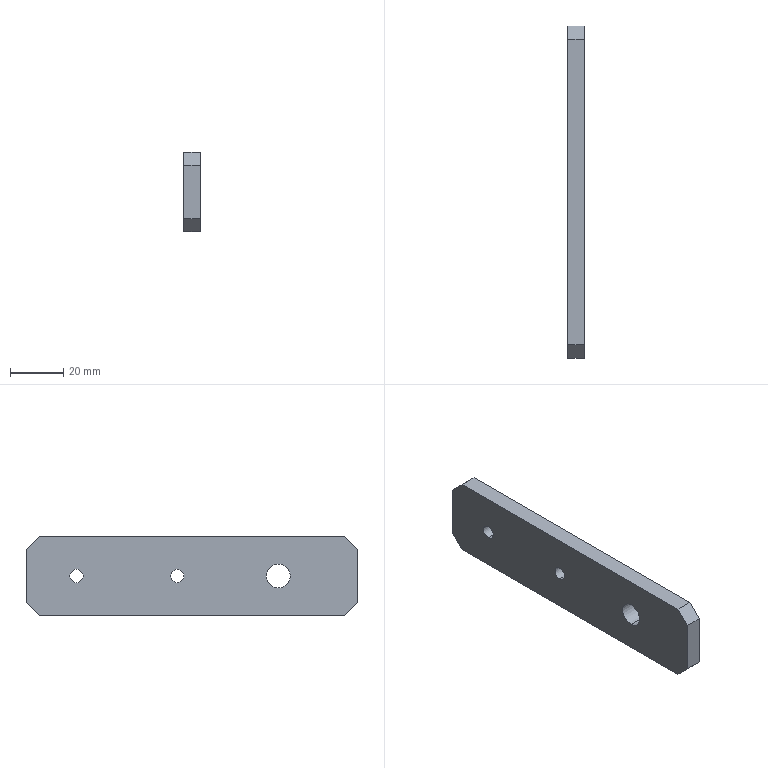Part | STEP file | PLACA SOPORTE GUIA | 1 solid | 16 faces | box 6.35 x 125 x 30 mm | volume 22842 mm3 | plane 10 | cylinder 6 | commonest cylinder face diameters 5 x4 9 x2
STEP:
#1=CARTESIAN_POINT('',(6.35,43.5,-2.5));
#2=VERTEX_POINT('',#1);
#3=CARTESIAN_POINT('',(6.35,43.5,2.5));
#4=VERTEX_POINT('',#3);
#5=CARTESIAN_POINT('',(6.35,43.5,0.));
#6=DIRECTION('',(-1.,0.,0.));
#7=DIRECTION('',(0.,0.,1.));
#8=AXIS2_PLACEMENT_3D('',#5,#6,#7);
#9=CIRCLE('',#8,2.5);
#10=EDGE_CURVE('',#2,#4,#9,.T.);
#11=ORIENTED_EDGE('',*,*,#10,.F.);
#12=CARTESIAN_POINT('',(0.,43.5,-2.5));
#13=VERTEX_POINT('',#12);
#14=CARTESIAN_POINT('',(0.,43.5,-2.5));
#15=DIRECTION('',(-1.,0.,0.));
#16=VECTOR('',#15,1000.);
#17=LINE('',#14,#16);
#18=EDGE_CURVE('',#2,#13,#17,.T.);
#19=ORIENTED_EDGE('',*,*,#18,.T.);
#20=CARTESIAN_POINT('',(0.,43.5,2.5));
#21=VERTEX_POINT('',#20);
#22=CARTESIAN_POINT('',(0.,43.5,0.));
#23=DIRECTION('',(-1.,0.,0.));
#24=DIRECTION('',(0.,0.,1.));
#25=AXIS2_PLACEMENT_3D('',#22,#23,#24);
#26=CIRCLE('',#25,2.5);
#27=EDGE_CURVE('',#13,#21,#26,.T.);
#28=ORIENTED_EDGE('',*,*,#27,.T.);
#29=CARTESIAN_POINT('',(0.,43.5,2.5));
#30=DIRECTION('',(-1.,0.,0.));
#31=VECTOR('',#30,1000.);
#32=LINE('',#29,#31);
#33=EDGE_CURVE('',#4,#21,#32,.T.);
#34=ORIENTED_EDGE('',*,*,#33,.F.);
#35=EDGE_LOOP('',(#11,#19,#28,#34));
#36=FACE_OUTER_BOUND('',#35,.T.);
#37=CARTESIAN_POINT('',(0.,43.5,0.));
#38=DIRECTION('',(-1.,0.,0.));
#39=DIRECTION('',(0.,0.,1.));
#40=AXIS2_PLACEMENT_3D('',#37,#38,#39);
#41=CYLINDRICAL_SURFACE('',#40,2.5);
#42=ADVANCED_FACE('',(#36),#41,.F.);
#43=CARTESIAN_POINT('',(6.35,5.5,-2.5));
#44=VERTEX_POINT('',#43);
#45=CARTESIAN_POINT('',(6.35,5.5,2.5));
#46=VERTEX_POINT('',#45);
#47=CARTESIAN_POINT('',(6.35,5.5,0.));
#48=DIRECTION('',(-1.,0.,0.));
#49=DIRECTION('',(0.,0.,1.));
#50=AXIS2_PLACEMENT_3D('',#47,#48,#49);
#51=CIRCLE('',#50,2.5);
#52=EDGE_CURVE('',#44,#46,#51,.T.);
#53=ORIENTED_EDGE('',*,*,#52,.F.);
#54=CARTESIAN_POINT('',(0.,5.5,-2.5));
#55=VERTEX_POINT('',#54);
#56=CARTESIAN_POINT('',(0.,5.5,-2.5));
#57=DIRECTION('',(-1.,0.,0.));
#58=VECTOR('',#57,1000.);
#59=LINE('',#56,#58);
#60=EDGE_CURVE('',#44,#55,#59,.T.);
#61=ORIENTED_EDGE('',*,*,#60,.T.);
#62=CARTESIAN_POINT('',(0.,5.5,2.5));
#63=VERTEX_POINT('',#62);
#64=CARTESIAN_POINT('',(0.,5.5,0.));
#65=DIRECTION('',(-1.,0.,0.));
#66=DIRECTION('',(0.,0.,1.));
#67=AXIS2_PLACEMENT_3D('',#64,#65,#66);
#68=CIRCLE('',#67,2.5);
#69=EDGE_CURVE('',#55,#63,#68,.T.);
#70=ORIENTED_EDGE('',*,*,#69,.T.);
#71=CARTESIAN_POINT('',(0.,5.5,2.5));
#72=DIRECTION('',(-1.,0.,0.));
#73=VECTOR('',#72,1000.);
#74=LINE('',#71,#73);
#75=EDGE_CURVE('',#46,#63,#74,.T.);
#76=ORIENTED_EDGE('',*,*,#75,.F.);
#77=EDGE_LOOP('',(#53,#61,#70,#76));
#78=FACE_OUTER_BOUND('',#77,.T.);
#79=CARTESIAN_POINT('',(0.,5.5,0.));
#80=DIRECTION('',(-1.,0.,0.));
#81=DIRECTION('',(0.,0.,1.));
#82=AXIS2_PLACEMENT_3D('',#79,#80,#81);
#83=CYLINDRICAL_SURFACE('',#82,2.5);
#84=ADVANCED_FACE('',(#78),#83,.F.);
#85=CARTESIAN_POINT('',(6.35,-32.5,-4.5));
#86=VERTEX_POINT('',#85);
#87=CARTESIAN_POINT('',(6.35,-32.5,4.5));
#88=VERTEX_POINT('',#87);
#89=CARTESIAN_POINT('',(6.35,-32.5,0.));
#90=DIRECTION('',(-1.,0.,0.));
#91=DIRECTION('',(0.,0.,1.));
#92=AXIS2_PLACEMENT_3D('',#89,#90,#91);
#93=CIRCLE('',#92,4.5);
#94=EDGE_CURVE('',#86,#88,#93,.T.);
#95=ORIENTED_EDGE('',*,*,#94,.F.);
#96=CARTESIAN_POINT('',(0.,-32.5,-4.5));
#97=VERTEX_POINT('',#96);
#98=CARTESIAN_POINT('',(0.,-32.5,-4.5));
#99=DIRECTION('',(-1.,0.,0.));
#100=VECTOR('',#99,1000.);
#101=LINE('',#98,#100);
#102=EDGE_CURVE('',#86,#97,#101,.T.);
#103=ORIENTED_EDGE('',*,*,#102,.T.);
#104=CARTESIAN_POINT('',(0.,-32.5,4.5));
#105=VERTEX_POINT('',#104);
#106=CARTESIAN_POINT('',(0.,-32.5,0.));
#107=DIRECTION('',(-1.,0.,0.));
#108=DIRECTION('',(0.,0.,1.));
#109=AXIS2_PLACEMENT_3D('',#106,#107,#108);
#110=CIRCLE('',#109,4.5);
#111=EDGE_CURVE('',#97,#105,#110,.T.);
#112=ORIENTED_EDGE('',*,*,#111,.T.);
#113=CARTESIAN_POINT('',(0.,-32.5,4.5));
#114=DIRECTION('',(-1.,0.,0.));
#115=VECTOR('',#114,1000.);
#116=LINE('',#113,#115);
#117=EDGE_CURVE('',#88,#105,#116,.T.);
#118=ORIENTED_EDGE('',*,*,#117,.F.);
#119=EDGE_LOOP('',(#95,#103,#112,#118));
#120=FACE_OUTER_BOUND('',#119,.T.);
#121=CARTESIAN_POINT('',(0.,-32.5,0.));
#122=DIRECTION('',(-1.,0.,0.));
#123=DIRECTION('',(0.,0.,1.));
#124=AXIS2_PLACEMENT_3D('',#121,#122,#123);
#125=CYLINDRICAL_SURFACE('',#124,4.5);
#126=ADVANCED_FACE('',(#120),#125,.F.);
#127=CARTESIAN_POINT('',(6.35,-57.5,-15.));
#128=VERTEX_POINT('',#127);
#129=CARTESIAN_POINT('',(6.35,57.5,-15.));
#130=VERTEX_POINT('',#129);
#131=CARTESIAN_POINT('',(6.35,62.5,-15.));
#132=DIRECTION('',(0.,1.,0.));
#133=VECTOR('',#132,1000.);
#134=LINE('',#131,#133);
#135=EDGE_CURVE('',#128,#130,#134,.T.);
#136=ORIENTED_EDGE('',*,*,#135,.F.);
#137=CARTESIAN_POINT('',(0.,-57.5,-15.));
#138=VERTEX_POINT('',#137);
#139=CARTESIAN_POINT('',(6.35,-57.5,-15.));
#140=DIRECTION('',(-1.,0.,0.));
#141=VECTOR('',#140,1000.);
#142=LINE('',#139,#141);
#143=EDGE_CURVE('',#128,#138,#142,.T.);
#144=ORIENTED_EDGE('',*,*,#143,.T.);
#145=CARTESIAN_POINT('',(0.,57.5,-15.));
#146=VERTEX_POINT('',#145);
#147=CARTESIAN_POINT('',(0.,62.5,-15.));
#148=DIRECTION('',(0.,1.,0.));
#149=VECTOR('',#148,1000.);
#150=LINE('',#147,#149);
#151=EDGE_CURVE('',#138,#146,#150,.T.);
#152=ORIENTED_EDGE('',*,*,#151,.T.);
#153=CARTESIAN_POINT('',(6.35,57.5,-15.));
#154=DIRECTION('',(1.,0.,0.));
#155=VECTOR('',#154,1000.);
#156=LINE('',#153,#155);
#157=EDGE_CURVE('',#146,#130,#156,.T.);
#158=ORIENTED_EDGE('',*,*,#157,.T.);
#159=EDGE_LOOP('',(#136,#144,#152,#158));
#160=FACE_OUTER_BOUND('',#159,.T.);
#161=CARTESIAN_POINT('',(6.35,62.5,-15.));
#162=DIRECTION('',(0.,0.,1.));
#163=DIRECTION('',(0.,-1.,0.));
#164=AXIS2_PLACEMENT_3D('',#161,#162,#163);
#165=PLANE('',#164);
#166=ADVANCED_FACE('',(#160),#165,.F.);
#167=CARTESIAN_POINT('',(6.35,62.5,-10.));
#168=VERTEX_POINT('',#167);
#169=CARTESIAN_POINT('',(6.35,62.5,10.));
#170=VERTEX_POINT('',#169);
#171=CARTESIAN_POINT('',(6.35,62.5,15.));
#172=DIRECTION('',(0.,0.,1.));
#173=VECTOR('',#172,1000.);
#174=LINE('',#171,#173);
#175=EDGE_CURVE('',#168,#170,#174,.T.);
#176=ORIENTED_EDGE('',*,*,#175,.F.);
#177=CARTESIAN_POINT('',(0.,62.5,-10.));
#178=VERTEX_POINT('',#177);
#179=CARTESIAN_POINT('',(6.35,62.5,-10.));
#180=DIRECTION('',(-1.,0.,0.));
#181=VECTOR('',#180,1000.);
#182=LINE('',#179,#181);
#183=EDGE_CURVE('',#168,#178,#182,.T.);
#184=ORIENTED_EDGE('',*,*,#183,.T.);
#185=CARTESIAN_POINT('',(0.,62.5,10.));
#186=VERTEX_POINT('',#185);
#187=CARTESIAN_POINT('',(0.,62.5,15.));
#188=DIRECTION('',(0.,0.,1.));
#189=VECTOR('',#188,1000.);
#190=LINE('',#187,#189);
#191=EDGE_CURVE('',#178,#186,#190,.T.);
#192=ORIENTED_EDGE('',*,*,#191,.T.);
#193=CARTESIAN_POINT('',(6.35,62.5,10.));
#194=DIRECTION('',(1.,0.,0.));
#195=VECTOR('',#194,1000.);
#196=LINE('',#193,#195);
#197=EDGE_CURVE('',#186,#170,#196,.T.);
#198=ORIENTED_EDGE('',*,*,#197,.T.);
#199=EDGE_LOOP('',(#176,#184,#192,#198));
#200=FACE_OUTER_BOUND('',#199,.T.);
#201=CARTESIAN_POINT('',(6.35,62.5,15.));
#202=DIRECTION('',(0.,-1.,0.));
#203=DIRECTION('',(0.,0.,-1.));
#204=AXIS2_PLACEMENT_3D('',#201,#202,#203);
#205=PLANE('',#204);
#206=ADVANCED_FACE('',(#200),#205,.F.);
#207=CARTESIAN_POINT('',(0.,57.5,15.));
#208=VERTEX_POINT('',#207);
#209=CARTESIAN_POINT('',(0.,-57.5,15.));
#210=VERTEX_POINT('',#209);
#211=CARTESIAN_POINT('',(0.,62.5,15.));
#212=DIRECTION('',(0.,-1.,0.));
#213=VECTOR('',#212,1000.);
#214=LINE('',#211,#213);
#215=EDGE_CURVE('',#208,#210,#214,.T.);
#216=ORIENTED_EDGE('',*,*,#215,.T.);
#217=CARTESIAN_POINT('',(6.35,-57.5,15.));
#218=VERTEX_POINT('',#217);
#219=CARTESIAN_POINT('',(6.35,-57.5,15.));
#220=DIRECTION('',(1.,0.,0.));
#221=VECTOR('',#220,1000.);
#222=LINE('',#219,#221);
#223=EDGE_CURVE('',#210,#218,#222,.T.);
#224=ORIENTED_EDGE('',*,*,#223,.T.);
#225=CARTESIAN_POINT('',(6.35,57.5,15.));
#226=VERTEX_POINT('',#225);
#227=CARTESIAN_POINT('',(6.35,62.5,15.));
#228=DIRECTION('',(0.,-1.,0.));
#229=VECTOR('',#228,1000.);
#230=LINE('',#227,#229);
#231=EDGE_CURVE('',#226,#218,#230,.T.);
#232=ORIENTED_EDGE('',*,*,#231,.F.);
#233=CARTESIAN_POINT('',(6.35,57.5,15.));
#234=DIRECTION('',(-1.,0.,0.));
#235=VECTOR('',#234,1000.);
#236=LINE('',#233,#235);
#237=EDGE_CURVE('',#226,#208,#236,.T.);
#238=ORIENTED_EDGE('',*,*,#237,.T.);
#239=EDGE_LOOP('',(#216,#224,#232,#238));
#240=FACE_OUTER_BOUND('',#239,.T.);
#241=CARTESIAN_POINT('',(6.35,62.5,15.));
#242=DIRECTION('',(0.,0.,-1.));
#243=DIRECTION('',(0.,1.,0.));
#244=AXIS2_PLACEMENT_3D('',#241,#242,#243);
#245=PLANE('',#244);
#246=ADVANCED_FACE('',(#240),#245,.F.);
#247=CARTESIAN_POINT('',(0.,-62.5,10.));
#248=VERTEX_POINT('',#247);
#249=CARTESIAN_POINT('',(0.,-62.5,-10.));
#250=VERTEX_POINT('',#249);
#251=CARTESIAN_POINT('',(0.,-62.5,15.));
#252=DIRECTION('',(0.,0.,-1.));
#253=VECTOR('',#252,1000.);
#254=LINE('',#251,#253);
#255=EDGE_CURVE('',#248,#250,#254,.T.);
#256=ORIENTED_EDGE('',*,*,#255,.T.);
#257=CARTESIAN_POINT('',(6.35,-62.5,-10.));
#258=VERTEX_POINT('',#257);
#259=CARTESIAN_POINT('',(6.35,-62.5,-10.));
#260=DIRECTION('',(1.,0.,0.));
#261=VECTOR('',#260,1000.);
#262=LINE('',#259,#261);
#263=EDGE_CURVE('',#250,#258,#262,.T.);
#264=ORIENTED_EDGE('',*,*,#263,.T.);
#265=CARTESIAN_POINT('',(6.35,-62.5,10.));
#266=VERTEX_POINT('',#265);
#267=CARTESIAN_POINT('',(6.35,-62.5,15.));
#268=DIRECTION('',(0.,0.,-1.));
#269=VECTOR('',#268,1000.);
#270=LINE('',#267,#269);
#271=EDGE_CURVE('',#266,#258,#270,.T.);
#272=ORIENTED_EDGE('',*,*,#271,.F.);
#273=CARTESIAN_POINT('',(6.35,-62.5,10.));
#274=DIRECTION('',(-1.,0.,0.));
#275=VECTOR('',#274,1000.);
#276=LINE('',#273,#275);
#277=EDGE_CURVE('',#266,#248,#276,.T.);
#278=ORIENTED_EDGE('',*,*,#277,.T.);
#279=EDGE_LOOP('',(#256,#264,#272,#278));
#280=FACE_OUTER_BOUND('',#279,.T.);
#281=CARTESIAN_POINT('',(6.35,-62.5,15.));
#282=DIRECTION('',(0.,1.,0.));
#283=DIRECTION('',(0.,0.,1.));
#284=AXIS2_PLACEMENT_3D('',#281,#282,#283);
#285=PLANE('',#284);
#286=ADVANCED_FACE('',(#280),#285,.F.);
#287=CARTESIAN_POINT('',(6.35,43.5,0.));
#288=DIRECTION('',(-1.,0.,0.));
#289=DIRECTION('',(0.,0.,1.));
#290=AXIS2_PLACEMENT_3D('',#287,#288,#289);
#291=CIRCLE('',#290,2.5);
#292=EDGE_CURVE('',#4,#2,#291,.T.);
#293=ORIENTED_EDGE('',*,*,#292,.T.);
#294=ORIENTED_EDGE('',*,*,#10,.T.);
#295=EDGE_LOOP('',(#293,#294));
#296=FACE_BOUND('',#295,.T.);
#297=CARTESIAN_POINT('',(6.35,5.5,0.));
#298=DIRECTION('',(-1.,0.,0.));
#299=DIRECTION('',(0.,0.,1.));
#300=AXIS2_PLACEMENT_3D('',#297,#298,#299);
#301=CIRCLE('',#300,2.5);
#302=EDGE_CURVE('',#46,#44,#301,.T.);
#303=ORIENTED_EDGE('',*,*,#302,.T.);
#304=ORIENTED_EDGE('',*,*,#52,.T.);
#305=EDGE_LOOP('',(#303,#304));
#306=FACE_BOUND('',#305,.T.);
#307=CARTESIAN_POINT('',(6.35,-32.5,0.));
#308=DIRECTION('',(-1.,0.,0.));
#309=DIRECTION('',(0.,0.,1.));
#310=AXIS2_PLACEMENT_3D('',#307,#308,#309);
#311=CIRCLE('',#310,4.5);
#312=EDGE_CURVE('',#88,#86,#311,.T.);
#313=ORIENTED_EDGE('',*,*,#312,.T.);
#314=ORIENTED_EDGE('',*,*,#94,.T.);
#315=EDGE_LOOP('',(#313,#314));
#316=FACE_BOUND('',#315,.T.);
#317=ORIENTED_EDGE('',*,*,#271,.T.);
#318=CARTESIAN_POINT('',(6.35,-36.25,-36.25));
#319=DIRECTION('',(0.,0.7071,-0.7071));
#320=VECTOR('',#319,1000.);
#321=LINE('',#318,#320);
#322=EDGE_CURVE('',#258,#128,#321,.T.);
#323=ORIENTED_EDGE('',*,*,#322,.T.);
#324=ORIENTED_EDGE('',*,*,#135,.T.);
#325=CARTESIAN_POINT('',(6.35,36.25,-36.25));
#326=DIRECTION('',(0.,0.7071,0.7071));
#327=VECTOR('',#326,1000.);
#328=LINE('',#325,#327);
#329=EDGE_CURVE('',#130,#168,#328,.T.);
#330=ORIENTED_EDGE('',*,*,#329,.T.);
#331=ORIENTED_EDGE('',*,*,#175,.T.);
#332=CARTESIAN_POINT('',(6.35,36.25,36.25));
#333=DIRECTION('',(0.,-0.7071,0.7071));
#334=VECTOR('',#333,1000.);
#335=LINE('',#332,#334);
#336=EDGE_CURVE('',#170,#226,#335,.T.);
#337=ORIENTED_EDGE('',*,*,#336,.T.);
#338=ORIENTED_EDGE('',*,*,#231,.T.);
#339=CARTESIAN_POINT('',(6.35,-36.25,36.25));
#340=DIRECTION('',(0.,-0.7071,-0.7071));
#341=VECTOR('',#340,1000.);
#342=LINE('',#339,#341);
#343=EDGE_CURVE('',#218,#266,#342,.T.);
#344=ORIENTED_EDGE('',*,*,#343,.T.);
#345=EDGE_LOOP('',(#317,#323,#324,#330,#331,#337,#338,#344));
#346=FACE_OUTER_BOUND('',#345,.T.);
#347=CARTESIAN_POINT('',(6.35,0.,0.));
#348=DIRECTION('',(1.,0.,0.));
#349=DIRECTION('',(0.,0.,-1.));
#350=AXIS2_PLACEMENT_3D('',#347,#348,#349);
#351=PLANE('',#350);
#352=ADVANCED_FACE('',(#296,#306,#316,#346),#351,.T.);
#353=CARTESIAN_POINT('',(0.,43.5,0.));
#354=DIRECTION('',(-1.,0.,0.));
#355=DIRECTION('',(0.,0.,1.));
#356=AXIS2_PLACEMENT_3D('',#353,#354,#355);
#357=CIRCLE('',#356,2.5);
#358=EDGE_CURVE('',#21,#13,#357,.T.);
#359=ORIENTED_EDGE('',*,*,#358,.F.);
#360=ORIENTED_EDGE('',*,*,#27,.F.);
#361=EDGE_LOOP('',(#359,#360));
#362=FACE_BOUND('',#361,.T.);
#363=CARTESIAN_POINT('',(0.,5.5,0.));
#364=DIRECTION('',(-1.,0.,0.));
#365=DIRECTION('',(0.,0.,1.));
#366=AXIS2_PLACEMENT_3D('',#363,#364,#365);
#367=CIRCLE('',#366,2.5);
#368=EDGE_CURVE('',#63,#55,#367,.T.);
#369=ORIENTED_EDGE('',*,*,#368,.F.);
#370=ORIENTED_EDGE('',*,*,#69,.F.);
#371=EDGE_LOOP('',(#369,#370));
#372=FACE_BOUND('',#371,.T.);
#373=CARTESIAN_POINT('',(0.,-32.5,0.));
#374=DIRECTION('',(-1.,0.,0.));
#375=DIRECTION('',(0.,0.,1.));
#376=AXIS2_PLACEMENT_3D('',#373,#374,#375);
#377=CIRCLE('',#376,4.5);
#378=EDGE_CURVE('',#105,#97,#377,.T.);
#379=ORIENTED_EDGE('',*,*,#378,.F.);
#380=ORIENTED_EDGE('',*,*,#111,.F.);
#381=EDGE_LOOP('',(#379,#380));
#382=FACE_BOUND('',#381,.T.);
#383=ORIENTED_EDGE('',*,*,#151,.F.);
#384=CARTESIAN_POINT('',(0.,-57.5,-15.));
#385=DIRECTION('',(0.,-0.7071,0.7071));
#386=VECTOR('',#385,1000.);
#387=LINE('',#384,#386);
#388=EDGE_CURVE('',#138,#250,#387,.T.);
#389=ORIENTED_EDGE('',*,*,#388,.T.);
#390=ORIENTED_EDGE('',*,*,#255,.F.);
#391=CARTESIAN_POINT('',(0.,-62.5,10.));
#392=DIRECTION('',(0.,0.7071,0.7071));
#393=VECTOR('',#392,1000.);
#394=LINE('',#391,#393);
#395=EDGE_CURVE('',#248,#210,#394,.T.);
#396=ORIENTED_EDGE('',*,*,#395,.T.);
#397=ORIENTED_EDGE('',*,*,#215,.F.);
#398=CARTESIAN_POINT('',(0.,57.5,15.));
#399=DIRECTION('',(0.,0.7071,-0.7071));
#400=VECTOR('',#399,1000.);
#401=LINE('',#398,#400);
#402=EDGE_CURVE('',#208,#186,#401,.T.);
#403=ORIENTED_EDGE('',*,*,#402,.T.);
#404=ORIENTED_EDGE('',*,*,#191,.F.);
#405=CARTESIAN_POINT('',(0.,62.5,-10.));
#406=DIRECTION('',(0.,-0.7071,-0.7071));
#407=VECTOR('',#406,1000.);
#408=LINE('',#405,#407);
#409=EDGE_CURVE('',#178,#146,#408,.T.);
#410=ORIENTED_EDGE('',*,*,#409,.T.);
#411=EDGE_LOOP('',(#383,#389,#390,#396,#397,#403,#404,#410));
#412=FACE_OUTER_BOUND('',#411,.T.);
#413=CARTESIAN_POINT('',(0.,0.,0.));
#414=DIRECTION('',(1.,0.,0.));
#415=DIRECTION('',(0.,0.,-1.));
#416=AXIS2_PLACEMENT_3D('',#413,#414,#415);
#417=PLANE('',#416);
#418=ADVANCED_FACE('',(#362,#372,#382,#412),#417,.F.);
#419=ORIENTED_EDGE('',*,*,#322,.F.);
#420=ORIENTED_EDGE('',*,*,#263,.F.);
#421=ORIENTED_EDGE('',*,*,#388,.F.);
#422=ORIENTED_EDGE('',*,*,#143,.F.);
#423=EDGE_LOOP('',(#419,#420,#421,#422));
#424=FACE_OUTER_BOUND('',#423,.T.);
#425=CARTESIAN_POINT('',(6.35,-57.5,-15.));
#426=DIRECTION('',(0.,0.7071,0.7071));
#427=DIRECTION('',(-1.,0.,0.));
#428=AXIS2_PLACEMENT_3D('',#425,#426,#427);
#429=PLANE('',#428);
#430=ADVANCED_FACE('',(#424),#429,.F.);
#431=ORIENTED_EDGE('',*,*,#343,.F.);
#432=ORIENTED_EDGE('',*,*,#223,.F.);
#433=ORIENTED_EDGE('',*,*,#395,.F.);
#434=ORIENTED_EDGE('',*,*,#277,.F.);
#435=EDGE_LOOP('',(#431,#432,#433,#434));
#436=FACE_OUTER_BOUND('',#435,.T.);
#437=CARTESIAN_POINT('',(6.35,-62.5,10.));
#438=DIRECTION('',(0.,0.7071,-0.7071));
#439=DIRECTION('',(-1.,0.,0.));
#440=AXIS2_PLACEMENT_3D('',#437,#438,#439);
#441=PLANE('',#440);
#442=ADVANCED_FACE('',(#436),#441,.F.);
#443=ORIENTED_EDGE('',*,*,#329,.F.);
#444=ORIENTED_EDGE('',*,*,#157,.F.);
#445=ORIENTED_EDGE('',*,*,#409,.F.);
#446=ORIENTED_EDGE('',*,*,#183,.F.);
#447=EDGE_LOOP('',(#443,#444,#445,#446));
#448=FACE_OUTER_BOUND('',#447,.T.);
#449=CARTESIAN_POINT('',(6.35,62.5,-10.));
#450=DIRECTION('',(0.,-0.7071,0.7071));
#451=DIRECTION('',(-1.,0.,0.));
#452=AXIS2_PLACEMENT_3D('',#449,#450,#451);
#453=PLANE('',#452);
#454=ADVANCED_FACE('',(#448),#453,.F.);
#455=ORIENTED_EDGE('',*,*,#336,.F.);
#456=ORIENTED_EDGE('',*,*,#197,.F.);
#457=ORIENTED_EDGE('',*,*,#402,.F.);
#458=ORIENTED_EDGE('',*,*,#237,.F.);
#459=EDGE_LOOP('',(#455,#456,#457,#458));
#460=FACE_OUTER_BOUND('',#459,.T.);
#461=CARTESIAN_POINT('',(6.35,57.5,15.));
#462=DIRECTION('',(0.,-0.7071,-0.7071));
#463=DIRECTION('',(-1.,0.,0.));
#464=AXIS2_PLACEMENT_3D('',#461,#462,#463);
#465=PLANE('',#464);
#466=ADVANCED_FACE('',(#460),#465,.F.);
#467=ORIENTED_EDGE('',*,*,#102,.F.);
#468=ORIENTED_EDGE('',*,*,#312,.F.);
#469=ORIENTED_EDGE('',*,*,#117,.T.);
#470=ORIENTED_EDGE('',*,*,#378,.T.);
#471=EDGE_LOOP('',(#467,#468,#469,#470));
#472=FACE_OUTER_BOUND('',#471,.T.);
#473=CARTESIAN_POINT('',(0.,-32.5,0.));
#474=DIRECTION('',(-1.,0.,0.));
#475=DIRECTION('',(0.,0.,1.));
#476=AXIS2_PLACEMENT_3D('',#473,#474,#475);
#477=CYLINDRICAL_SURFACE('',#476,4.5);
#478=ADVANCED_FACE('',(#472),#477,.F.);
#479=ORIENTED_EDGE('',*,*,#60,.F.);
#480=ORIENTED_EDGE('',*,*,#302,.F.);
#481=ORIENTED_EDGE('',*,*,#75,.T.);
#482=ORIENTED_EDGE('',*,*,#368,.T.);
#483=EDGE_LOOP('',(#479,#480,#481,#482));
#484=FACE_OUTER_BOUND('',#483,.T.);
#485=CARTESIAN_POINT('',(0.,5.5,0.));
#486=DIRECTION('',(-1.,0.,0.));
#487=DIRECTION('',(0.,0.,1.));
#488=AXIS2_PLACEMENT_3D('',#485,#486,#487);
#489=CYLINDRICAL_SURFACE('',#488,2.5);
#490=ADVANCED_FACE('',(#484),#489,.F.);
#491=ORIENTED_EDGE('',*,*,#18,.F.);
#492=ORIENTED_EDGE('',*,*,#292,.F.);
#493=ORIENTED_EDGE('',*,*,#33,.T.);
#494=ORIENTED_EDGE('',*,*,#358,.T.);
#495=EDGE_LOOP('',(#491,#492,#493,#494));
#496=FACE_OUTER_BOUND('',#495,.T.);
#497=CARTESIAN_POINT('',(0.,43.5,0.));
#498=DIRECTION('',(-1.,0.,0.));
#499=DIRECTION('',(0.,0.,1.));
#500=AXIS2_PLACEMENT_3D('',#497,#498,#499);
#501=CYLINDRICAL_SURFACE('',#500,2.5);
#502=ADVANCED_FACE('',(#496),#501,.F.);
#503=CLOSED_SHELL('',(#42,#84,#126,#166,#206,#246,#286,#352,#418,#430,#442,#454,#466,#478,#490,#502));
#504=MANIFOLD_SOLID_BREP('',#503);
#505=CARTESIAN_POINT('',(0.,0.,0.));
#506=DIRECTION('',(0.,0.,1.));
#507=DIRECTION('',(1.,0.,0.));
#508=AXIS2_PLACEMENT_3D('',#505,#506,#507);
#509=(LENGTH_UNIT()NAMED_UNIT(*)SI_UNIT(.MILLI.,.METRE.));
#510=UNCERTAINTY_MEASURE_WITH_UNIT(LENGTH_MEASURE(0.00001),#509,'','');
#511=(NAMED_UNIT(*)PLANE_ANGLE_UNIT()SI_UNIT($,.RADIAN.));
#512=(NAMED_UNIT(*)SI_UNIT($,.STERADIAN.)SOLID_ANGLE_UNIT());
#513=(GEOMETRIC_REPRESENTATION_CONTEXT(3)GLOBAL_UNCERTAINTY_ASSIGNED_CONTEXT((#510))GLOBAL_UNIT_ASSIGNED_CONTEXT((#509,#511,#512))REPRESENTATION_CONTEXT('',''));
#514=ADVANCED_BREP_SHAPE_REPRESENTATION('',(#504,#508),#513);